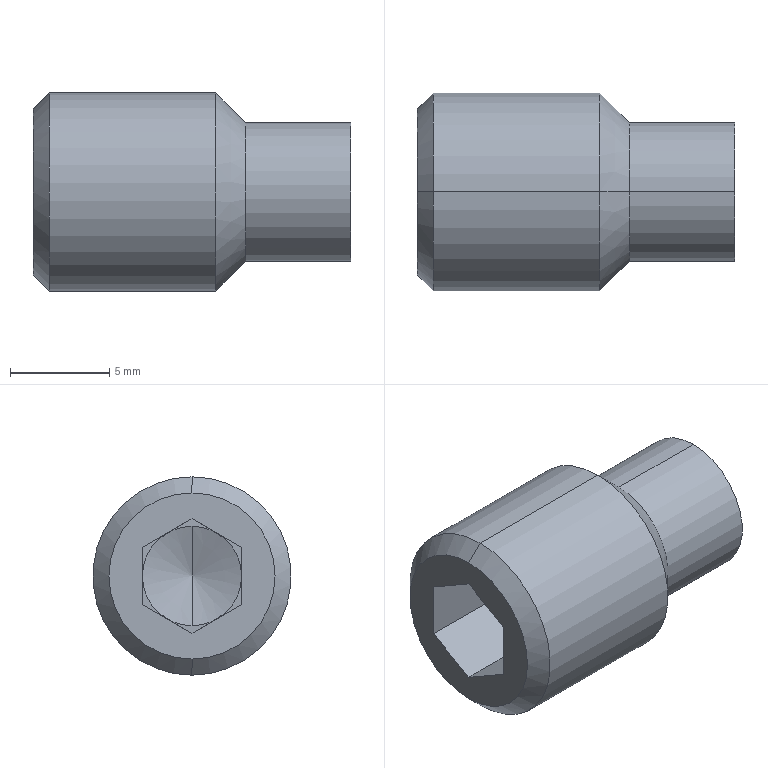Part | SolidWorks | features RevCut 2, Cut 1, LPattern 1, Revolution 1 | 1 solid | 24 faces | box 16 x 10 x 10 mm | volume 910.9 mm3 | plane 14 | cone 6 | cylinder 4 | commonest cylinder face diameters 7 x2 10 x2
STEP:
#1=CARTESIAN_POINT('',(4.8,0.,0.));
#2=VERTEX_POINT('',#1);
#3=CARTESIAN_POINT('',(4.,0.,2.5));
#4=VERTEX_POINT('',#3);
#5=CARTESIAN_POINT('',(4.8,0.,0.));
#6=DIRECTION('',(-0.3048,0.,0.9524));
#7=VECTOR('',#6,1000.);
#8=LINE('',#5,#7);
#9=EDGE_CURVE('',#2,#4,#8,.T.);
#10=ORIENTED_EDGE('',*,*,#9,.F.);
#11=CARTESIAN_POINT('',(4.,0.,-2.5));
#12=VERTEX_POINT('',#11);
#13=CARTESIAN_POINT('',(4.8,0.,0.));
#14=DIRECTION('',(-0.3048,0.,-0.9524));
#15=VECTOR('',#14,1000.);
#16=LINE('',#13,#15);
#17=EDGE_CURVE('',#2,#12,#16,.T.);
#18=ORIENTED_EDGE('',*,*,#17,.T.);
#19=CARTESIAN_POINT('',(4.,-1.25,-2.165));
#20=VERTEX_POINT('',#19);
#21=CARTESIAN_POINT('',(4.,0.,0.));
#22=DIRECTION('',(-1.,0.,0.));
#23=DIRECTION('',(0.,0.,1.));
#24=AXIS2_PLACEMENT_3D('',#21,#22,#23);
#25=CIRCLE('',#24,2.5);
#26=EDGE_CURVE('',#12,#20,#25,.T.);
#27=ORIENTED_EDGE('',*,*,#26,.T.);
#28=CARTESIAN_POINT('',(4.,-2.5,0.));
#29=VERTEX_POINT('',#28);
#30=CARTESIAN_POINT('',(4.,0.,0.));
#31=DIRECTION('',(-1.,0.,0.));
#32=DIRECTION('',(0.,0.,1.));
#33=AXIS2_PLACEMENT_3D('',#30,#31,#32);
#34=CIRCLE('',#33,2.5);
#35=EDGE_CURVE('',#20,#29,#34,.T.);
#36=ORIENTED_EDGE('',*,*,#35,.T.);
#37=CARTESIAN_POINT('',(4.,-1.25,2.165));
#38=VERTEX_POINT('',#37);
#39=CARTESIAN_POINT('',(4.,0.,0.));
#40=DIRECTION('',(-1.,0.,0.));
#41=DIRECTION('',(0.,0.,1.));
#42=AXIS2_PLACEMENT_3D('',#39,#40,#41);
#43=CIRCLE('',#42,2.5);
#44=EDGE_CURVE('',#29,#38,#43,.T.);
#45=ORIENTED_EDGE('',*,*,#44,.T.);
#46=CARTESIAN_POINT('',(4.,0.,0.));
#47=DIRECTION('',(-1.,0.,0.));
#48=DIRECTION('',(0.,0.,1.));
#49=AXIS2_PLACEMENT_3D('',#46,#47,#48);
#50=CIRCLE('',#49,2.5);
#51=EDGE_CURVE('',#38,#4,#50,.T.);
#52=ORIENTED_EDGE('',*,*,#51,.T.);
#53=EDGE_LOOP('',(#10,#18,#27,#36,#45,#52));
#54=FACE_OUTER_BOUND('',#53,.T.);
#55=CARTESIAN_POINT('',(-995.2,0.,0.));
#56=DIRECTION('',(-1.,0.,0.));
#57=DIRECTION('',(0.,0.,1.));
#58=AXIS2_PLACEMENT_3D('',#55,#56,#57);
#59=CONICAL_SURFACE('',#58,3125.,1.261);
#60=ADVANCED_FACE('',(#54),#59,.F.);
#61=CARTESIAN_POINT('',(0.,0.,4.188));
#62=VERTEX_POINT('',#61);
#63=CARTESIAN_POINT('',(0.,0.,-4.188));
#64=VERTEX_POINT('',#63);
#65=CARTESIAN_POINT('',(0.,0.,0.));
#66=DIRECTION('',(-1.,0.,0.));
#67=DIRECTION('',(0.,0.,1.));
#68=AXIS2_PLACEMENT_3D('',#65,#66,#67);
#69=CIRCLE('',#68,4.188);
#70=EDGE_CURVE('',#62,#64,#69,.T.);
#71=ORIENTED_EDGE('',*,*,#70,.F.);
#72=CARTESIAN_POINT('',(0.812,0.,5.));
#73=VERTEX_POINT('',#72);
#74=CARTESIAN_POINT('',(0.812,0.,5.));
#75=DIRECTION('',(0.7071,0.,0.7071));
#76=VECTOR('',#75,1000.);
#77=LINE('',#74,#76);
#78=EDGE_CURVE('',#62,#73,#77,.T.);
#79=ORIENTED_EDGE('',*,*,#78,.T.);
#80=CARTESIAN_POINT('',(0.812,0.,-5.));
#81=VERTEX_POINT('',#80);
#82=CARTESIAN_POINT('',(0.812,0.,0.));
#83=DIRECTION('',(-1.,0.,0.));
#84=DIRECTION('',(0.,0.,1.));
#85=AXIS2_PLACEMENT_3D('',#82,#83,#84);
#86=CIRCLE('',#85,5.);
#87=EDGE_CURVE('',#73,#81,#86,.T.);
#88=ORIENTED_EDGE('',*,*,#87,.T.);
#89=CARTESIAN_POINT('',(0.812,0.,-5.));
#90=DIRECTION('',(0.7071,0.,-0.7071));
#91=VECTOR('',#90,1000.);
#92=LINE('',#89,#91);
#93=EDGE_CURVE('',#64,#81,#92,.T.);
#94=ORIENTED_EDGE('',*,*,#93,.F.);
#95=EDGE_LOOP('',(#71,#79,#88,#94));
#96=FACE_OUTER_BOUND('',#95,.T.);
#97=CARTESIAN_POINT('',(0.812,0.,0.));
#98=DIRECTION('',(1.,0.,0.));
#99=DIRECTION('',(0.,0.,-1.));
#100=AXIS2_PLACEMENT_3D('',#97,#98,#99);
#101=CONICAL_SURFACE('',#100,5.,0.7854);
#102=ADVANCED_FACE('',(#96),#101,.T.);
#103=CARTESIAN_POINT('',(9.2,0.,5.));
#104=VERTEX_POINT('',#103);
#105=CARTESIAN_POINT('',(9.2,0.,-5.));
#106=VERTEX_POINT('',#105);
#107=CARTESIAN_POINT('',(9.2,0.,0.));
#108=DIRECTION('',(-1.,0.,0.));
#109=DIRECTION('',(0.,0.,1.));
#110=AXIS2_PLACEMENT_3D('',#107,#108,#109);
#111=CIRCLE('',#110,5.);
#112=EDGE_CURVE('',#104,#106,#111,.T.);
#113=ORIENTED_EDGE('',*,*,#112,.T.);
#114=CARTESIAN_POINT('',(-1.969,0.,-5.));
#115=DIRECTION('',(-1.,0.,0.));
#116=VECTOR('',#115,1000.);
#117=LINE('',#114,#116);
#118=EDGE_CURVE('',#106,#81,#117,.T.);
#119=ORIENTED_EDGE('',*,*,#118,.T.);
#120=ORIENTED_EDGE('',*,*,#87,.F.);
#121=CARTESIAN_POINT('',(-1.969,0.,5.));
#122=DIRECTION('',(-1.,0.,0.));
#123=VECTOR('',#122,1000.);
#124=LINE('',#121,#123);
#125=EDGE_CURVE('',#104,#73,#124,.T.);
#126=ORIENTED_EDGE('',*,*,#125,.F.);
#127=EDGE_LOOP('',(#113,#119,#120,#126));
#128=FACE_OUTER_BOUND('',#127,.T.);
#129=CARTESIAN_POINT('',(-1.969,0.,0.));
#130=DIRECTION('',(-1.,0.,0.));
#131=DIRECTION('',(0.,0.,1.));
#132=AXIS2_PLACEMENT_3D('',#129,#130,#131);
#133=CYLINDRICAL_SURFACE('',#132,5.);
#134=ADVANCED_FACE('',(#128),#133,.T.);
#135=CARTESIAN_POINT('',(10.7,0.,3.5));
#136=VERTEX_POINT('',#135);
#137=CARTESIAN_POINT('',(10.7,0.,-3.5));
#138=VERTEX_POINT('',#137);
#139=CARTESIAN_POINT('',(10.7,0.,0.));
#140=DIRECTION('',(-1.,0.,0.));
#141=DIRECTION('',(0.,0.,1.));
#142=AXIS2_PLACEMENT_3D('',#139,#140,#141);
#143=CIRCLE('',#142,3.5);
#144=EDGE_CURVE('',#136,#138,#143,.T.);
#145=ORIENTED_EDGE('',*,*,#144,.T.);
#146=CARTESIAN_POINT('',(10.7,0.,-3.5));
#147=DIRECTION('',(-0.7071,0.,-0.7071));
#148=VECTOR('',#147,1000.);
#149=LINE('',#146,#148);
#150=EDGE_CURVE('',#138,#106,#149,.T.);
#151=ORIENTED_EDGE('',*,*,#150,.T.);
#152=ORIENTED_EDGE('',*,*,#112,.F.);
#153=CARTESIAN_POINT('',(10.7,0.,3.5));
#154=DIRECTION('',(-0.7071,0.,0.7071));
#155=VECTOR('',#154,1000.);
#156=LINE('',#153,#155);
#157=EDGE_CURVE('',#136,#104,#156,.T.);
#158=ORIENTED_EDGE('',*,*,#157,.F.);
#159=EDGE_LOOP('',(#145,#151,#152,#158));
#160=FACE_OUTER_BOUND('',#159,.T.);
#161=CARTESIAN_POINT('',(10.7,0.,0.));
#162=DIRECTION('',(-1.,0.,0.));
#163=DIRECTION('',(0.,0.,1.));
#164=AXIS2_PLACEMENT_3D('',#161,#162,#163);
#165=CONICAL_SURFACE('',#164,3.5,0.7854);
#166=ADVANCED_FACE('',(#160),#165,.T.);
#167=CARTESIAN_POINT('',(16.,0.,3.5));
#168=VERTEX_POINT('',#167);
#169=CARTESIAN_POINT('',(16.,0.,-3.5));
#170=VERTEX_POINT('',#169);
#171=CARTESIAN_POINT('',(16.,0.,0.));
#172=DIRECTION('',(-1.,0.,0.));
#173=DIRECTION('',(0.,0.,1.));
#174=AXIS2_PLACEMENT_3D('',#171,#172,#173);
#175=CIRCLE('',#174,3.5);
#176=EDGE_CURVE('',#168,#170,#175,.T.);
#177=ORIENTED_EDGE('',*,*,#176,.T.);
#178=CARTESIAN_POINT('',(-1.969,0.,-3.5));
#179=DIRECTION('',(-1.,0.,0.));
#180=VECTOR('',#179,1000.);
#181=LINE('',#178,#180);
#182=EDGE_CURVE('',#170,#138,#181,.T.);
#183=ORIENTED_EDGE('',*,*,#182,.T.);
#184=ORIENTED_EDGE('',*,*,#144,.F.);
#185=CARTESIAN_POINT('',(-1.969,0.,3.5));
#186=DIRECTION('',(-1.,0.,0.));
#187=VECTOR('',#186,1000.);
#188=LINE('',#185,#187);
#189=EDGE_CURVE('',#168,#136,#188,.T.);
#190=ORIENTED_EDGE('',*,*,#189,.F.);
#191=EDGE_LOOP('',(#177,#183,#184,#190));
#192=FACE_OUTER_BOUND('',#191,.T.);
#193=CARTESIAN_POINT('',(-1.969,0.,0.));
#194=DIRECTION('',(-1.,0.,0.));
#195=DIRECTION('',(0.,0.,1.));
#196=AXIS2_PLACEMENT_3D('',#193,#194,#195);
#197=CYLINDRICAL_SURFACE('',#196,3.5);
#198=ADVANCED_FACE('',(#192),#197,.T.);
#199=CARTESIAN_POINT('',(4.,1.25,2.165));
#200=VERTEX_POINT('',#199);
#201=CARTESIAN_POINT('',(4.,2.5,0.));
#202=VERTEX_POINT('',#201);
#203=CARTESIAN_POINT('',(4.,0.,0.));
#204=DIRECTION('',(-1.,0.,0.));
#205=DIRECTION('',(0.,0.,1.));
#206=AXIS2_PLACEMENT_3D('',#203,#204,#205);
#207=CIRCLE('',#206,2.5);
#208=EDGE_CURVE('',#200,#202,#207,.T.);
#209=ORIENTED_EDGE('',*,*,#208,.F.);
#210=CARTESIAN_POINT('',(4.,2.5,1.443));
#211=VERTEX_POINT('',#210);
#212=CARTESIAN_POINT('',(4.,0.,2.887));
#213=DIRECTION('',(0.,0.866,-0.5));
#214=VECTOR('',#213,1000.);
#215=LINE('',#212,#214);
#216=EDGE_CURVE('',#200,#211,#215,.T.);
#217=ORIENTED_EDGE('',*,*,#216,.T.);
#218=CARTESIAN_POINT('',(4.,2.5,1.443));
#219=DIRECTION('',(0.,0.,-1.));
#220=VECTOR('',#219,1000.);
#221=LINE('',#218,#220);
#222=EDGE_CURVE('',#211,#202,#221,.T.);
#223=ORIENTED_EDGE('',*,*,#222,.T.);
#224=EDGE_LOOP('',(#209,#217,#223));
#225=FACE_OUTER_BOUND('',#224,.T.);
#226=CARTESIAN_POINT('',(4.,0.,2.887));
#227=DIRECTION('',(-1.,0.,0.));
#228=DIRECTION('',(0.,0.,1.));
#229=AXIS2_PLACEMENT_3D('',#226,#227,#228);
#230=PLANE('',#229);
#231=ADVANCED_FACE('',(#225),#230,.T.);
#232=CARTESIAN_POINT('',(4.,1.25,-2.165));
#233=VERTEX_POINT('',#232);
#234=CARTESIAN_POINT('',(4.,0.,0.));
#235=DIRECTION('',(-1.,0.,0.));
#236=DIRECTION('',(0.,0.,1.));
#237=AXIS2_PLACEMENT_3D('',#234,#235,#236);
#238=CIRCLE('',#237,2.5);
#239=EDGE_CURVE('',#202,#233,#238,.T.);
#240=ORIENTED_EDGE('',*,*,#239,.F.);
#241=CARTESIAN_POINT('',(4.,2.5,-1.443));
#242=VERTEX_POINT('',#241);
#243=CARTESIAN_POINT('',(4.,2.5,1.443));
#244=DIRECTION('',(0.,0.,-1.));
#245=VECTOR('',#244,1000.);
#246=LINE('',#243,#245);
#247=EDGE_CURVE('',#202,#242,#246,.T.);
#248=ORIENTED_EDGE('',*,*,#247,.T.);
#249=CARTESIAN_POINT('',(4.,2.5,-1.443));
#250=DIRECTION('',(0.,-0.866,-0.5));
#251=VECTOR('',#250,1000.);
#252=LINE('',#249,#251);
#253=EDGE_CURVE('',#242,#233,#252,.T.);
#254=ORIENTED_EDGE('',*,*,#253,.T.);
#255=EDGE_LOOP('',(#240,#248,#254));
#256=FACE_OUTER_BOUND('',#255,.T.);
#257=CARTESIAN_POINT('',(4.,0.,2.887));
#258=DIRECTION('',(-1.,0.,0.));
#259=DIRECTION('',(0.,0.,1.));
#260=AXIS2_PLACEMENT_3D('',#257,#258,#259);
#261=PLANE('',#260);
#262=ADVANCED_FACE('',(#256),#261,.T.);
#263=CARTESIAN_POINT('',(4.,0.,0.));
#264=DIRECTION('',(-1.,0.,0.));
#265=DIRECTION('',(0.,0.,1.));
#266=AXIS2_PLACEMENT_3D('',#263,#264,#265);
#267=CIRCLE('',#266,2.5);
#268=EDGE_CURVE('',#233,#12,#267,.T.);
#269=ORIENTED_EDGE('',*,*,#268,.F.);
#270=CARTESIAN_POINT('',(4.,0.,-2.887));
#271=VERTEX_POINT('',#270);
#272=CARTESIAN_POINT('',(4.,2.5,-1.443));
#273=DIRECTION('',(0.,-0.866,-0.5));
#274=VECTOR('',#273,1000.);
#275=LINE('',#272,#274);
#276=EDGE_CURVE('',#233,#271,#275,.T.);
#277=ORIENTED_EDGE('',*,*,#276,.T.);
#278=CARTESIAN_POINT('',(4.,0.,-2.887));
#279=DIRECTION('',(0.,-0.866,0.5));
#280=VECTOR('',#279,1000.);
#281=LINE('',#278,#280);
#282=EDGE_CURVE('',#271,#20,#281,.T.);
#283=ORIENTED_EDGE('',*,*,#282,.T.);
#284=ORIENTED_EDGE('',*,*,#26,.F.);
#285=EDGE_LOOP('',(#269,#277,#283,#284));
#286=FACE_OUTER_BOUND('',#285,.T.);
#287=CARTESIAN_POINT('',(4.,0.,2.887));
#288=DIRECTION('',(-1.,0.,0.));
#289=DIRECTION('',(0.,0.,1.));
#290=AXIS2_PLACEMENT_3D('',#287,#288,#289);
#291=PLANE('',#290);
#292=ADVANCED_FACE('',(#286),#291,.T.);
#293=ORIENTED_EDGE('',*,*,#35,.F.);
#294=CARTESIAN_POINT('',(4.,-2.5,-1.443));
#295=VERTEX_POINT('',#294);
#296=CARTESIAN_POINT('',(4.,0.,-2.887));
#297=DIRECTION('',(0.,-0.866,0.5));
#298=VECTOR('',#297,1000.);
#299=LINE('',#296,#298);
#300=EDGE_CURVE('',#20,#295,#299,.T.);
#301=ORIENTED_EDGE('',*,*,#300,.T.);
#302=CARTESIAN_POINT('',(4.,-2.5,-1.443));
#303=DIRECTION('',(0.,0.,1.));
#304=VECTOR('',#303,1000.);
#305=LINE('',#302,#304);
#306=EDGE_CURVE('',#295,#29,#305,.T.);
#307=ORIENTED_EDGE('',*,*,#306,.T.);
#308=EDGE_LOOP('',(#293,#301,#307));
#309=FACE_OUTER_BOUND('',#308,.T.);
#310=CARTESIAN_POINT('',(4.,0.,2.887));
#311=DIRECTION('',(-1.,0.,0.));
#312=DIRECTION('',(0.,0.,1.));
#313=AXIS2_PLACEMENT_3D('',#310,#311,#312);
#314=PLANE('',#313);
#315=ADVANCED_FACE('',(#309),#314,.T.);
#316=ORIENTED_EDGE('',*,*,#44,.F.);
#317=CARTESIAN_POINT('',(4.,-2.5,1.443));
#318=VERTEX_POINT('',#317);
#319=CARTESIAN_POINT('',(4.,-2.5,-1.443));
#320=DIRECTION('',(0.,0.,1.));
#321=VECTOR('',#320,1000.);
#322=LINE('',#319,#321);
#323=EDGE_CURVE('',#29,#318,#322,.T.);
#324=ORIENTED_EDGE('',*,*,#323,.T.);
#325=CARTESIAN_POINT('',(4.,-2.5,1.443));
#326=DIRECTION('',(0.,0.866,0.5));
#327=VECTOR('',#326,1000.);
#328=LINE('',#325,#327);
#329=EDGE_CURVE('',#318,#38,#328,.T.);
#330=ORIENTED_EDGE('',*,*,#329,.T.);
#331=EDGE_LOOP('',(#316,#324,#330));
#332=FACE_OUTER_BOUND('',#331,.T.);
#333=CARTESIAN_POINT('',(4.,0.,2.887));
#334=DIRECTION('',(-1.,0.,0.));
#335=DIRECTION('',(0.,0.,1.));
#336=AXIS2_PLACEMENT_3D('',#333,#334,#335);
#337=PLANE('',#336);
#338=ADVANCED_FACE('',(#332),#337,.T.);
#339=CARTESIAN_POINT('',(0.,0.,2.887));
#340=VERTEX_POINT('',#339);
#341=CARTESIAN_POINT('',(0.,2.5,1.443));
#342=VERTEX_POINT('',#341);
#343=CARTESIAN_POINT('',(0.,0.,2.887));
#344=DIRECTION('',(0.,0.866,-0.5));
#345=VECTOR('',#344,1000.);
#346=LINE('',#343,#345);
#347=EDGE_CURVE('',#340,#342,#346,.T.);
#348=ORIENTED_EDGE('',*,*,#347,.F.);
#349=CARTESIAN_POINT('',(0.,-2.5,1.443));
#350=VERTEX_POINT('',#349);
#351=CARTESIAN_POINT('',(0.,-2.5,1.443));
#352=DIRECTION('',(0.,0.866,0.5));
#353=VECTOR('',#352,1000.);
#354=LINE('',#351,#353);
#355=EDGE_CURVE('',#350,#340,#354,.T.);
#356=ORIENTED_EDGE('',*,*,#355,.F.);
#357=CARTESIAN_POINT('',(0.,-2.5,-1.443));
#358=VERTEX_POINT('',#357);
#359=CARTESIAN_POINT('',(0.,-2.5,-1.443));
#360=DIRECTION('',(0.,0.,1.));
#361=VECTOR('',#360,1000.);
#362=LINE('',#359,#361);
#363=EDGE_CURVE('',#358,#350,#362,.T.);
#364=ORIENTED_EDGE('',*,*,#363,.F.);
#365=CARTESIAN_POINT('',(0.,0.,-2.887));
#366=VERTEX_POINT('',#365);
#367=CARTESIAN_POINT('',(0.,0.,-2.887));
#368=DIRECTION('',(0.,-0.866,0.5));
#369=VECTOR('',#368,1000.);
#370=LINE('',#367,#369);
#371=EDGE_CURVE('',#366,#358,#370,.T.);
#372=ORIENTED_EDGE('',*,*,#371,.F.);
#373=CARTESIAN_POINT('',(0.,2.5,-1.443));
#374=VERTEX_POINT('',#373);
#375=CARTESIAN_POINT('',(0.,2.5,-1.443));
#376=DIRECTION('',(0.,-0.866,-0.5));
#377=VECTOR('',#376,1000.);
#378=LINE('',#375,#377);
#379=EDGE_CURVE('',#374,#366,#378,.T.);
#380=ORIENTED_EDGE('',*,*,#379,.F.);
#381=CARTESIAN_POINT('',(0.,2.5,1.443));
#382=DIRECTION('',(0.,0.,-1.));
#383=VECTOR('',#382,1000.);
#384=LINE('',#381,#383);
#385=EDGE_CURVE('',#342,#374,#384,.T.);
#386=ORIENTED_EDGE('',*,*,#385,.F.);
#387=EDGE_LOOP('',(#348,#356,#364,#372,#380,#386));
#388=FACE_BOUND('',#387,.T.);
#389=CARTESIAN_POINT('',(0.,0.,0.));
#390=DIRECTION('',(-1.,0.,0.));
#391=DIRECTION('',(0.,0.,1.));
#392=AXIS2_PLACEMENT_3D('',#389,#390,#391);
#393=CIRCLE('',#392,4.188);
#394=EDGE_CURVE('',#64,#62,#393,.T.);
#395=ORIENTED_EDGE('',*,*,#394,.T.);
#396=ORIENTED_EDGE('',*,*,#70,.T.);
#397=EDGE_LOOP('',(#395,#396));
#398=FACE_OUTER_BOUND('',#397,.T.);
#399=CARTESIAN_POINT('',(0.,4.188,0.));
#400=DIRECTION('',(1.,0.,0.));
#401=DIRECTION('',(0.,0.,-1.));
#402=AXIS2_PLACEMENT_3D('',#399,#400,#401);
#403=PLANE('',#402);
#404=ADVANCED_FACE('',(#388,#398),#403,.F.);
#405=ORIENTED_EDGE('',*,*,#176,.F.);
#406=CARTESIAN_POINT('',(16.,0.,0.));
#407=DIRECTION('',(-1.,0.,0.));
#408=DIRECTION('',(0.,0.,1.));
#409=AXIS2_PLACEMENT_3D('',#406,#407,#408);
#410=CIRCLE('',#409,3.5);
#411=EDGE_CURVE('',#170,#168,#410,.T.);
#412=ORIENTED_EDGE('',*,*,#411,.F.);
#413=EDGE_LOOP('',(#405,#412));
#414=FACE_OUTER_BOUND('',#413,.T.);
#415=CARTESIAN_POINT('',(16.,0.,0.));
#416=DIRECTION('',(-1.,0.,0.));
#417=DIRECTION('',(0.,0.,1.));
#418=AXIS2_PLACEMENT_3D('',#415,#416,#417);
#419=PLANE('',#418);
#420=ADVANCED_FACE('',(#414),#419,.F.);
#421=ORIENTED_EDGE('',*,*,#182,.F.);
#422=ORIENTED_EDGE('',*,*,#411,.T.);
#423=ORIENTED_EDGE('',*,*,#189,.T.);
#424=CARTESIAN_POINT('',(10.7,0.,0.));
#425=DIRECTION('',(-1.,0.,0.));
#426=DIRECTION('',(0.,0.,1.));
#427=AXIS2_PLACEMENT_3D('',#424,#425,#426);
#428=CIRCLE('',#427,3.5);
#429=EDGE_CURVE('',#138,#136,#428,.T.);
#430=ORIENTED_EDGE('',*,*,#429,.F.);
#431=EDGE_LOOP('',(#421,#422,#423,#430));
#432=FACE_OUTER_BOUND('',#431,.T.);
#433=CARTESIAN_POINT('',(-1.969,0.,0.));
#434=DIRECTION('',(-1.,0.,0.));
#435=DIRECTION('',(0.,0.,1.));
#436=AXIS2_PLACEMENT_3D('',#433,#434,#435);
#437=CYLINDRICAL_SURFACE('',#436,3.5);
#438=ADVANCED_FACE('',(#432),#437,.T.);
#439=ORIENTED_EDGE('',*,*,#150,.F.);
#440=ORIENTED_EDGE('',*,*,#429,.T.);
#441=ORIENTED_EDGE('',*,*,#157,.T.);
#442=CARTESIAN_POINT('',(9.2,0.,0.));
#443=DIRECTION('',(-1.,0.,0.));
#444=DIRECTION('',(0.,0.,1.));
#445=AXIS2_PLACEMENT_3D('',#442,#443,#444);
#446=CIRCLE('',#445,5.);
#447=EDGE_CURVE('',#106,#104,#446,.T.);
#448=ORIENTED_EDGE('',*,*,#447,.F.);
#449=EDGE_LOOP('',(#439,#440,#441,#448));
#450=FACE_OUTER_BOUND('',#449,.T.);
#451=CARTESIAN_POINT('',(10.7,0.,0.));
#452=DIRECTION('',(-1.,0.,0.));
#453=DIRECTION('',(0.,0.,1.));
#454=AXIS2_PLACEMENT_3D('',#451,#452,#453);
#455=CONICAL_SURFACE('',#454,3.5,0.7854);
#456=ADVANCED_FACE('',(#450),#455,.T.);
#457=ORIENTED_EDGE('',*,*,#118,.F.);
#458=ORIENTED_EDGE('',*,*,#447,.T.);
#459=ORIENTED_EDGE('',*,*,#125,.T.);
#460=CARTESIAN_POINT('',(0.812,0.,0.));
#461=DIRECTION('',(-1.,0.,0.));
#462=DIRECTION('',(0.,0.,1.));
#463=AXIS2_PLACEMENT_3D('',#460,#461,#462);
#464=CIRCLE('',#463,5.);
#465=EDGE_CURVE('',#81,#73,#464,.T.);
#466=ORIENTED_EDGE('',*,*,#465,.F.);
#467=EDGE_LOOP('',(#457,#458,#459,#466));
#468=FACE_OUTER_BOUND('',#467,.T.);
#469=CARTESIAN_POINT('',(-1.969,0.,0.));
#470=DIRECTION('',(-1.,0.,0.));
#471=DIRECTION('',(0.,0.,1.));
#472=AXIS2_PLACEMENT_3D('',#469,#470,#471);
#473=CYLINDRICAL_SURFACE('',#472,5.);
#474=ADVANCED_FACE('',(#468),#473,.T.);
#475=ORIENTED_EDGE('',*,*,#78,.F.);
#476=ORIENTED_EDGE('',*,*,#394,.F.);
#477=ORIENTED_EDGE('',*,*,#93,.T.);
#478=ORIENTED_EDGE('',*,*,#465,.T.);
#479=EDGE_LOOP('',(#475,#476,#477,#478));
#480=FACE_OUTER_BOUND('',#479,.T.);
#481=CARTESIAN_POINT('',(0.812,0.,0.));
#482=DIRECTION('',(1.,0.,0.));
#483=DIRECTION('',(0.,0.,-1.));
#484=AXIS2_PLACEMENT_3D('',#481,#482,#483);
#485=CONICAL_SURFACE('',#484,5.,0.7854);
#486=ADVANCED_FACE('',(#480),#485,.T.);
#487=ORIENTED_EDGE('',*,*,#355,.T.);
#488=CARTESIAN_POINT('',(4.,0.,2.887));
#489=VERTEX_POINT('',#488);
#490=CARTESIAN_POINT('',(4.,0.,2.887));
#491=DIRECTION('',(-1.,0.,0.));
#492=VECTOR('',#491,1000.);
#493=LINE('',#490,#492);
#494=EDGE_CURVE('',#489,#340,#493,.T.);
#495=ORIENTED_EDGE('',*,*,#494,.F.);
#496=CARTESIAN_POINT('',(4.,-2.5,1.443));
#497=DIRECTION('',(0.,0.866,0.5));
#498=VECTOR('',#497,1000.);
#499=LINE('',#496,#498);
#500=EDGE_CURVE('',#38,#489,#499,.T.);
#501=ORIENTED_EDGE('',*,*,#500,.F.);
#502=ORIENTED_EDGE('',*,*,#329,.F.);
#503=CARTESIAN_POINT('',(4.,-2.5,1.443));
#504=DIRECTION('',(-1.,0.,0.));
#505=VECTOR('',#504,1000.);
#506=LINE('',#503,#505);
#507=EDGE_CURVE('',#318,#350,#506,.T.);
#508=ORIENTED_EDGE('',*,*,#507,.T.);
#509=EDGE_LOOP('',(#487,#495,#501,#502,#508));
#510=FACE_OUTER_BOUND('',#509,.T.);
#511=CARTESIAN_POINT('',(4.,-2.5,1.443));
#512=DIRECTION('',(0.,-0.5,0.866));
#513=DIRECTION('',(0.,-0.866,-0.5));
#514=AXIS2_PLACEMENT_3D('',#511,#512,#513);
#515=PLANE('',#514);
#516=ADVANCED_FACE('',(#510),#515,.F.);
#517=ORIENTED_EDGE('',*,*,#363,.T.);
#518=ORIENTED_EDGE('',*,*,#507,.F.);
#519=ORIENTED_EDGE('',*,*,#323,.F.);
#520=ORIENTED_EDGE('',*,*,#306,.F.);
#521=CARTESIAN_POINT('',(4.,-2.5,-1.443));
#522=DIRECTION('',(-1.,0.,0.));
#523=VECTOR('',#522,1000.);
#524=LINE('',#521,#523);
#525=EDGE_CURVE('',#295,#358,#524,.T.);
#526=ORIENTED_EDGE('',*,*,#525,.T.);
#527=EDGE_LOOP('',(#517,#518,#519,#520,#526));
#528=FACE_OUTER_BOUND('',#527,.T.);
#529=CARTESIAN_POINT('',(4.,-2.5,-1.443));
#530=DIRECTION('',(0.,-1.,0.));
#531=DIRECTION('',(0.,0.,-1.));
#532=AXIS2_PLACEMENT_3D('',#529,#530,#531);
#533=PLANE('',#532);
#534=ADVANCED_FACE('',(#528),#533,.F.);
#535=ORIENTED_EDGE('',*,*,#371,.T.);
#536=ORIENTED_EDGE('',*,*,#525,.F.);
#537=ORIENTED_EDGE('',*,*,#300,.F.);
#538=ORIENTED_EDGE('',*,*,#282,.F.);
#539=CARTESIAN_POINT('',(4.,0.,-2.887));
#540=DIRECTION('',(-1.,0.,0.));
#541=VECTOR('',#540,1000.);
#542=LINE('',#539,#541);
#543=EDGE_CURVE('',#271,#366,#542,.T.);
#544=ORIENTED_EDGE('',*,*,#543,.T.);
#545=EDGE_LOOP('',(#535,#536,#537,#538,#544));
#546=FACE_OUTER_BOUND('',#545,.T.);
#547=CARTESIAN_POINT('',(4.,0.,-2.887));
#548=DIRECTION('',(0.,-0.5,-0.866));
#549=DIRECTION('',(0.,0.866,-0.5));
#550=AXIS2_PLACEMENT_3D('',#547,#548,#549);
#551=PLANE('',#550);
#552=ADVANCED_FACE('',(#546),#551,.F.);
#553=ORIENTED_EDGE('',*,*,#379,.T.);
#554=ORIENTED_EDGE('',*,*,#543,.F.);
#555=ORIENTED_EDGE('',*,*,#276,.F.);
#556=ORIENTED_EDGE('',*,*,#253,.F.);
#557=CARTESIAN_POINT('',(4.,2.5,-1.443));
#558=DIRECTION('',(-1.,0.,0.));
#559=VECTOR('',#558,1000.);
#560=LINE('',#557,#559);
#561=EDGE_CURVE('',#242,#374,#560,.T.);
#562=ORIENTED_EDGE('',*,*,#561,.T.);
#563=EDGE_LOOP('',(#553,#554,#555,#556,#562));
#564=FACE_OUTER_BOUND('',#563,.T.);
#565=CARTESIAN_POINT('',(4.,2.5,-1.443));
#566=DIRECTION('',(0.,0.5,-0.866));
#567=DIRECTION('',(0.,0.866,0.5));
#568=AXIS2_PLACEMENT_3D('',#565,#566,#567);
#569=PLANE('',#568);
#570=ADVANCED_FACE('',(#564),#569,.F.);
#571=ORIENTED_EDGE('',*,*,#385,.T.);
#572=ORIENTED_EDGE('',*,*,#561,.F.);
#573=ORIENTED_EDGE('',*,*,#247,.F.);
#574=ORIENTED_EDGE('',*,*,#222,.F.);
#575=CARTESIAN_POINT('',(4.,2.5,1.443));
#576=DIRECTION('',(-1.,0.,0.));
#577=VECTOR('',#576,1000.);
#578=LINE('',#575,#577);
#579=EDGE_CURVE('',#211,#342,#578,.T.);
#580=ORIENTED_EDGE('',*,*,#579,.T.);
#581=EDGE_LOOP('',(#571,#572,#573,#574,#580));
#582=FACE_OUTER_BOUND('',#581,.T.);
#583=CARTESIAN_POINT('',(4.,2.5,1.443));
#584=DIRECTION('',(0.,1.,0.));
#585=DIRECTION('',(0.,0.,1.));
#586=AXIS2_PLACEMENT_3D('',#583,#584,#585);
#587=PLANE('',#586);
#588=ADVANCED_FACE('',(#582),#587,.F.);
#589=ORIENTED_EDGE('',*,*,#347,.T.);
#590=ORIENTED_EDGE('',*,*,#579,.F.);
#591=ORIENTED_EDGE('',*,*,#216,.F.);
#592=CARTESIAN_POINT('',(4.,0.,2.887));
#593=DIRECTION('',(0.,0.866,-0.5));
#594=VECTOR('',#593,1000.);
#595=LINE('',#592,#594);
#596=EDGE_CURVE('',#489,#200,#595,.T.);
#597=ORIENTED_EDGE('',*,*,#596,.F.);
#598=ORIENTED_EDGE('',*,*,#494,.T.);
#599=EDGE_LOOP('',(#589,#590,#591,#597,#598));
#600=FACE_OUTER_BOUND('',#599,.T.);
#601=CARTESIAN_POINT('',(4.,0.,2.887));
#602=DIRECTION('',(0.,0.5,0.866));
#603=DIRECTION('',(0.,-0.866,0.5));
#604=AXIS2_PLACEMENT_3D('',#601,#602,#603);
#605=PLANE('',#604);
#606=ADVANCED_FACE('',(#600),#605,.F.);
#607=ORIENTED_EDGE('',*,*,#51,.F.);
#608=ORIENTED_EDGE('',*,*,#500,.T.);
#609=ORIENTED_EDGE('',*,*,#596,.T.);
#610=CARTESIAN_POINT('',(4.,0.,0.));
#611=DIRECTION('',(-1.,0.,0.));
#612=DIRECTION('',(0.,0.,1.));
#613=AXIS2_PLACEMENT_3D('',#610,#611,#612);
#614=CIRCLE('',#613,2.5);
#615=EDGE_CURVE('',#4,#200,#614,.T.);
#616=ORIENTED_EDGE('',*,*,#615,.F.);
#617=EDGE_LOOP('',(#607,#608,#609,#616));
#618=FACE_OUTER_BOUND('',#617,.T.);
#619=CARTESIAN_POINT('',(4.,0.,2.887));
#620=DIRECTION('',(-1.,0.,0.));
#621=DIRECTION('',(0.,0.,1.));
#622=AXIS2_PLACEMENT_3D('',#619,#620,#621);
#623=PLANE('',#622);
#624=ADVANCED_FACE('',(#618),#623,.T.);
#625=ORIENTED_EDGE('',*,*,#17,.F.);
#626=ORIENTED_EDGE('',*,*,#9,.T.);
#627=ORIENTED_EDGE('',*,*,#615,.T.);
#628=ORIENTED_EDGE('',*,*,#208,.T.);
#629=ORIENTED_EDGE('',*,*,#239,.T.);
#630=ORIENTED_EDGE('',*,*,#268,.T.);
#631=EDGE_LOOP('',(#625,#626,#627,#628,#629,#630));
#632=FACE_OUTER_BOUND('',#631,.T.);
#633=CARTESIAN_POINT('',(-995.2,0.,0.));
#634=DIRECTION('',(-1.,0.,0.));
#635=DIRECTION('',(0.,0.,1.));
#636=AXIS2_PLACEMENT_3D('',#633,#634,#635);
#637=CONICAL_SURFACE('',#636,3125.,1.261);
#638=ADVANCED_FACE('',(#632),#637,.F.);
#639=CLOSED_SHELL('',(#60,#102,#134,#166,#198,#231,#262,#292,#315,#338,#404,#420,#438,#456,#474,#486,#516,#534,#552,#570,#588,#606,#624,#638));
#640=MANIFOLD_SOLID_BREP('',#639);
#641=CARTESIAN_POINT('',(0.,0.,0.));
#642=DIRECTION('',(0.,0.,1.));
#643=DIRECTION('',(1.,0.,0.));
#644=AXIS2_PLACEMENT_3D('',#641,#642,#643);
#645=(LENGTH_UNIT()NAMED_UNIT(*)SI_UNIT(.MILLI.,.METRE.));
#646=UNCERTAINTY_MEASURE_WITH_UNIT(LENGTH_MEASURE(0.00001),#645,'','');
#647=(NAMED_UNIT(*)PLANE_ANGLE_UNIT()SI_UNIT($,.RADIAN.));
#648=(NAMED_UNIT(*)SI_UNIT($,.STERADIAN.)SOLID_ANGLE_UNIT());
#649=(GEOMETRIC_REPRESENTATION_CONTEXT(3)GLOBAL_UNCERTAINTY_ASSIGNED_CONTEXT((#646))GLOBAL_UNIT_ASSIGNED_CONTEXT((#645,#647,#648))REPRESENTATION_CONTEXT('',''));
#650=ADVANCED_BREP_SHAPE_REPRESENTATION('',(#640,#644),#649);